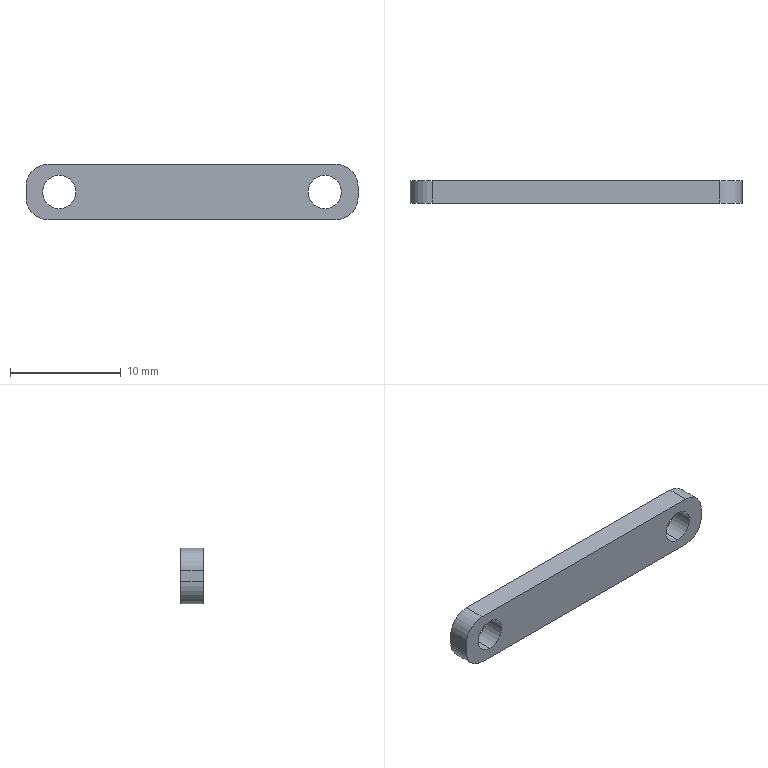Part | SolidWorks | features Extrusion 1 | 1 solid | 14 faces | box 30 x 2 x 5 mm | volume 264.858 mm3 | cylinder 8 | plane 6 | commonest cylinder face diameters 3 x4 4 x4
STEP:
#1=CARTESIAN_POINT('',(-12.,2.,-1.5));
#2=VERTEX_POINT('',#1);
#3=CARTESIAN_POINT('',(-12.,2.,1.5));
#4=VERTEX_POINT('',#3);
#5=CARTESIAN_POINT('',(-12.,2.,0.));
#6=DIRECTION('',(0.,1.,0.));
#7=DIRECTION('',(0.,0.,1.));
#8=AXIS2_PLACEMENT_3D('',#5,#6,#7);
#9=CIRCLE('',#8,1.5);
#10=EDGE_CURVE('',#2,#4,#9,.T.);
#11=ORIENTED_EDGE('',*,*,#10,.T.);
#12=CARTESIAN_POINT('',(-12.,0.,1.5));
#13=VERTEX_POINT('',#12);
#14=CARTESIAN_POINT('',(-12.,2.,1.5));
#15=DIRECTION('',(0.,-1.,0.));
#16=VECTOR('',#15,1000.);
#17=LINE('',#14,#16);
#18=EDGE_CURVE('',#4,#13,#17,.T.);
#19=ORIENTED_EDGE('',*,*,#18,.T.);
#20=CARTESIAN_POINT('',(-12.,0.,-1.5));
#21=VERTEX_POINT('',#20);
#22=CARTESIAN_POINT('',(-12.,0.,0.));
#23=DIRECTION('',(0.,1.,0.));
#24=DIRECTION('',(0.,0.,1.));
#25=AXIS2_PLACEMENT_3D('',#22,#23,#24);
#26=CIRCLE('',#25,1.5);
#27=EDGE_CURVE('',#21,#13,#26,.T.);
#28=ORIENTED_EDGE('',*,*,#27,.F.);
#29=CARTESIAN_POINT('',(-12.,2.,-1.5));
#30=DIRECTION('',(0.,-1.,0.));
#31=VECTOR('',#30,1000.);
#32=LINE('',#29,#31);
#33=EDGE_CURVE('',#2,#21,#32,.T.);
#34=ORIENTED_EDGE('',*,*,#33,.F.);
#35=EDGE_LOOP('',(#11,#19,#28,#34));
#36=FACE_OUTER_BOUND('',#35,.T.);
#37=CARTESIAN_POINT('',(-12.,2.,0.));
#38=DIRECTION('',(0.,-1.,0.));
#39=DIRECTION('',(0.,0.,-1.));
#40=AXIS2_PLACEMENT_3D('',#37,#38,#39);
#41=CYLINDRICAL_SURFACE('',#40,1.5);
#42=ADVANCED_FACE('',(#36),#41,.F.);
#43=CARTESIAN_POINT('',(12.,2.,-1.5));
#44=VERTEX_POINT('',#43);
#45=CARTESIAN_POINT('',(12.,2.,1.5));
#46=VERTEX_POINT('',#45);
#47=CARTESIAN_POINT('',(12.,2.,0.));
#48=DIRECTION('',(0.,1.,0.));
#49=DIRECTION('',(0.,0.,1.));
#50=AXIS2_PLACEMENT_3D('',#47,#48,#49);
#51=CIRCLE('',#50,1.5);
#52=EDGE_CURVE('',#44,#46,#51,.T.);
#53=ORIENTED_EDGE('',*,*,#52,.T.);
#54=CARTESIAN_POINT('',(12.,0.,1.5));
#55=VERTEX_POINT('',#54);
#56=CARTESIAN_POINT('',(12.,2.,1.5));
#57=DIRECTION('',(0.,-1.,0.));
#58=VECTOR('',#57,1000.);
#59=LINE('',#56,#58);
#60=EDGE_CURVE('',#46,#55,#59,.T.);
#61=ORIENTED_EDGE('',*,*,#60,.T.);
#62=CARTESIAN_POINT('',(12.,0.,-1.5));
#63=VERTEX_POINT('',#62);
#64=CARTESIAN_POINT('',(12.,0.,0.));
#65=DIRECTION('',(0.,1.,0.));
#66=DIRECTION('',(0.,0.,1.));
#67=AXIS2_PLACEMENT_3D('',#64,#65,#66);
#68=CIRCLE('',#67,1.5);
#69=EDGE_CURVE('',#63,#55,#68,.T.);
#70=ORIENTED_EDGE('',*,*,#69,.F.);
#71=CARTESIAN_POINT('',(12.,2.,-1.5));
#72=DIRECTION('',(0.,-1.,0.));
#73=VECTOR('',#72,1000.);
#74=LINE('',#71,#73);
#75=EDGE_CURVE('',#44,#63,#74,.T.);
#76=ORIENTED_EDGE('',*,*,#75,.F.);
#77=EDGE_LOOP('',(#53,#61,#70,#76));
#78=FACE_OUTER_BOUND('',#77,.T.);
#79=CARTESIAN_POINT('',(12.,2.,0.));
#80=DIRECTION('',(0.,-1.,0.));
#81=DIRECTION('',(0.,0.,-1.));
#82=AXIS2_PLACEMENT_3D('',#79,#80,#81);
#83=CYLINDRICAL_SURFACE('',#82,1.5);
#84=ADVANCED_FACE('',(#78),#83,.F.);
#85=ORIENTED_EDGE('',*,*,#52,.F.);
#86=CARTESIAN_POINT('',(12.,2.,0.));
#87=DIRECTION('',(0.,1.,0.));
#88=DIRECTION('',(0.,0.,1.));
#89=AXIS2_PLACEMENT_3D('',#86,#87,#88);
#90=CIRCLE('',#89,1.5);
#91=EDGE_CURVE('',#46,#44,#90,.T.);
#92=ORIENTED_EDGE('',*,*,#91,.F.);
#93=EDGE_LOOP('',(#85,#92));
#94=FACE_BOUND('',#93,.T.);
#95=CARTESIAN_POINT('',(15.,2.,-0.5));
#96=VERTEX_POINT('',#95);
#97=CARTESIAN_POINT('',(13.,2.,-2.5));
#98=VERTEX_POINT('',#97);
#99=CARTESIAN_POINT('',(13.,2.,-0.5));
#100=DIRECTION('',(0.,1.,0.));
#101=DIRECTION('',(0.,0.,1.));
#102=AXIS2_PLACEMENT_3D('',#99,#100,#101);
#103=CIRCLE('',#102,2.);
#104=EDGE_CURVE('',#96,#98,#103,.T.);
#105=ORIENTED_EDGE('',*,*,#104,.T.);
#106=CARTESIAN_POINT('',(-13.,2.,-2.5));
#107=VERTEX_POINT('',#106);
#108=CARTESIAN_POINT('',(-13.,2.,-2.5));
#109=DIRECTION('',(-1.,0.,0.));
#110=VECTOR('',#109,1000.);
#111=LINE('',#108,#110);
#112=EDGE_CURVE('',#98,#107,#111,.T.);
#113=ORIENTED_EDGE('',*,*,#112,.T.);
#114=CARTESIAN_POINT('',(-15.,2.,-0.5));
#115=VERTEX_POINT('',#114);
#116=CARTESIAN_POINT('',(-13.,2.,-0.5));
#117=DIRECTION('',(0.,1.,0.));
#118=DIRECTION('',(0.,0.,-1.));
#119=AXIS2_PLACEMENT_3D('',#116,#117,#118);
#120=CIRCLE('',#119,2.);
#121=EDGE_CURVE('',#107,#115,#120,.T.);
#122=ORIENTED_EDGE('',*,*,#121,.T.);
#123=CARTESIAN_POINT('',(-15.,2.,0.5));
#124=VERTEX_POINT('',#123);
#125=CARTESIAN_POINT('',(-15.,2.,0.5));
#126=DIRECTION('',(0.,0.,1.));
#127=VECTOR('',#126,1000.);
#128=LINE('',#125,#127);
#129=EDGE_CURVE('',#115,#124,#128,.T.);
#130=ORIENTED_EDGE('',*,*,#129,.T.);
#131=CARTESIAN_POINT('',(-13.,2.,2.5));
#132=VERTEX_POINT('',#131);
#133=CARTESIAN_POINT('',(-13.,2.,0.5));
#134=DIRECTION('',(0.,1.,0.));
#135=DIRECTION('',(0.,0.,-1.));
#136=AXIS2_PLACEMENT_3D('',#133,#134,#135);
#137=CIRCLE('',#136,2.);
#138=EDGE_CURVE('',#124,#132,#137,.T.);
#139=ORIENTED_EDGE('',*,*,#138,.T.);
#140=CARTESIAN_POINT('',(13.,2.,2.5));
#141=VERTEX_POINT('',#140);
#142=CARTESIAN_POINT('',(-13.,2.,2.5));
#143=DIRECTION('',(1.,0.,0.));
#144=VECTOR('',#143,1000.);
#145=LINE('',#142,#144);
#146=EDGE_CURVE('',#132,#141,#145,.T.);
#147=ORIENTED_EDGE('',*,*,#146,.T.);
#148=CARTESIAN_POINT('',(15.,2.,0.5));
#149=VERTEX_POINT('',#148);
#150=CARTESIAN_POINT('',(13.,2.,0.5));
#151=DIRECTION('',(0.,1.,0.));
#152=DIRECTION('',(0.,0.,-1.));
#153=AXIS2_PLACEMENT_3D('',#150,#151,#152);
#154=CIRCLE('',#153,2.);
#155=EDGE_CURVE('',#141,#149,#154,.T.);
#156=ORIENTED_EDGE('',*,*,#155,.T.);
#157=CARTESIAN_POINT('',(15.,2.,0.5));
#158=DIRECTION('',(0.,0.,-1.));
#159=VECTOR('',#158,1000.);
#160=LINE('',#157,#159);
#161=EDGE_CURVE('',#149,#96,#160,.T.);
#162=ORIENTED_EDGE('',*,*,#161,.T.);
#163=EDGE_LOOP('',(#105,#113,#122,#130,#139,#147,#156,#162));
#164=FACE_OUTER_BOUND('',#163,.T.);
#165=ORIENTED_EDGE('',*,*,#10,.F.);
#166=CARTESIAN_POINT('',(-12.,2.,0.));
#167=DIRECTION('',(0.,1.,0.));
#168=DIRECTION('',(0.,0.,1.));
#169=AXIS2_PLACEMENT_3D('',#166,#167,#168);
#170=CIRCLE('',#169,1.5);
#171=EDGE_CURVE('',#4,#2,#170,.T.);
#172=ORIENTED_EDGE('',*,*,#171,.F.);
#173=EDGE_LOOP('',(#165,#172));
#174=FACE_BOUND('',#173,.T.);
#175=CARTESIAN_POINT('',(13.,2.,-0.5));
#176=DIRECTION('',(0.,1.,0.));
#177=DIRECTION('',(0.,0.,1.));
#178=AXIS2_PLACEMENT_3D('',#175,#176,#177);
#179=PLANE('',#178);
#180=ADVANCED_FACE('',(#94,#164,#174),#179,.T.);
#181=CARTESIAN_POINT('',(15.,0.,-0.5));
#182=VERTEX_POINT('',#181);
#183=CARTESIAN_POINT('',(13.,0.,-2.5));
#184=VERTEX_POINT('',#183);
#185=CARTESIAN_POINT('',(13.,0.,-0.5));
#186=DIRECTION('',(0.,1.,0.));
#187=DIRECTION('',(0.,0.,1.));
#188=AXIS2_PLACEMENT_3D('',#185,#186,#187);
#189=CIRCLE('',#188,2.);
#190=EDGE_CURVE('',#182,#184,#189,.T.);
#191=ORIENTED_EDGE('',*,*,#190,.F.);
#192=CARTESIAN_POINT('',(15.,0.,0.5));
#193=VERTEX_POINT('',#192);
#194=CARTESIAN_POINT('',(15.,0.,0.5));
#195=DIRECTION('',(0.,0.,-1.));
#196=VECTOR('',#195,1000.);
#197=LINE('',#194,#196);
#198=EDGE_CURVE('',#193,#182,#197,.T.);
#199=ORIENTED_EDGE('',*,*,#198,.F.);
#200=CARTESIAN_POINT('',(13.,0.,2.5));
#201=VERTEX_POINT('',#200);
#202=CARTESIAN_POINT('',(13.,0.,0.5));
#203=DIRECTION('',(0.,1.,0.));
#204=DIRECTION('',(0.,0.,-1.));
#205=AXIS2_PLACEMENT_3D('',#202,#203,#204);
#206=CIRCLE('',#205,2.);
#207=EDGE_CURVE('',#201,#193,#206,.T.);
#208=ORIENTED_EDGE('',*,*,#207,.F.);
#209=CARTESIAN_POINT('',(-13.,0.,2.5));
#210=VERTEX_POINT('',#209);
#211=CARTESIAN_POINT('',(-13.,0.,2.5));
#212=DIRECTION('',(1.,0.,0.));
#213=VECTOR('',#212,1000.);
#214=LINE('',#211,#213);
#215=EDGE_CURVE('',#210,#201,#214,.T.);
#216=ORIENTED_EDGE('',*,*,#215,.F.);
#217=CARTESIAN_POINT('',(-15.,0.,0.5));
#218=VERTEX_POINT('',#217);
#219=CARTESIAN_POINT('',(-13.,0.,0.5));
#220=DIRECTION('',(0.,1.,0.));
#221=DIRECTION('',(0.,0.,-1.));
#222=AXIS2_PLACEMENT_3D('',#219,#220,#221);
#223=CIRCLE('',#222,2.);
#224=EDGE_CURVE('',#218,#210,#223,.T.);
#225=ORIENTED_EDGE('',*,*,#224,.F.);
#226=CARTESIAN_POINT('',(-15.,0.,-0.5));
#227=VERTEX_POINT('',#226);
#228=CARTESIAN_POINT('',(-15.,0.,0.5));
#229=DIRECTION('',(0.,0.,1.));
#230=VECTOR('',#229,1000.);
#231=LINE('',#228,#230);
#232=EDGE_CURVE('',#227,#218,#231,.T.);
#233=ORIENTED_EDGE('',*,*,#232,.F.);
#234=CARTESIAN_POINT('',(-13.,0.,-2.5));
#235=VERTEX_POINT('',#234);
#236=CARTESIAN_POINT('',(-13.,0.,-0.5));
#237=DIRECTION('',(0.,1.,0.));
#238=DIRECTION('',(0.,0.,-1.));
#239=AXIS2_PLACEMENT_3D('',#236,#237,#238);
#240=CIRCLE('',#239,2.);
#241=EDGE_CURVE('',#235,#227,#240,.T.);
#242=ORIENTED_EDGE('',*,*,#241,.F.);
#243=CARTESIAN_POINT('',(-13.,0.,-2.5));
#244=DIRECTION('',(-1.,0.,0.));
#245=VECTOR('',#244,1000.);
#246=LINE('',#243,#245);
#247=EDGE_CURVE('',#184,#235,#246,.T.);
#248=ORIENTED_EDGE('',*,*,#247,.F.);
#249=EDGE_LOOP('',(#191,#199,#208,#216,#225,#233,#242,#248));
#250=FACE_OUTER_BOUND('',#249,.T.);
#251=ORIENTED_EDGE('',*,*,#69,.T.);
#252=CARTESIAN_POINT('',(12.,0.,0.));
#253=DIRECTION('',(0.,1.,0.));
#254=DIRECTION('',(0.,0.,1.));
#255=AXIS2_PLACEMENT_3D('',#252,#253,#254);
#256=CIRCLE('',#255,1.5);
#257=EDGE_CURVE('',#55,#63,#256,.T.);
#258=ORIENTED_EDGE('',*,*,#257,.T.);
#259=EDGE_LOOP('',(#251,#258));
#260=FACE_BOUND('',#259,.T.);
#261=ORIENTED_EDGE('',*,*,#27,.T.);
#262=CARTESIAN_POINT('',(-12.,0.,0.));
#263=DIRECTION('',(0.,1.,0.));
#264=DIRECTION('',(0.,0.,1.));
#265=AXIS2_PLACEMENT_3D('',#262,#263,#264);
#266=CIRCLE('',#265,1.5);
#267=EDGE_CURVE('',#13,#21,#266,.T.);
#268=ORIENTED_EDGE('',*,*,#267,.T.);
#269=EDGE_LOOP('',(#261,#268));
#270=FACE_BOUND('',#269,.T.);
#271=CARTESIAN_POINT('',(13.,0.,-0.5));
#272=DIRECTION('',(0.,1.,0.));
#273=DIRECTION('',(0.,0.,1.));
#274=AXIS2_PLACEMENT_3D('',#271,#272,#273);
#275=PLANE('',#274);
#276=ADVANCED_FACE('',(#250,#260,#270),#275,.F.);
#277=ORIENTED_EDGE('',*,*,#190,.T.);
#278=CARTESIAN_POINT('',(13.,2.,-2.5));
#279=DIRECTION('',(0.,-1.,0.));
#280=VECTOR('',#279,1000.);
#281=LINE('',#278,#280);
#282=EDGE_CURVE('',#98,#184,#281,.T.);
#283=ORIENTED_EDGE('',*,*,#282,.F.);
#284=ORIENTED_EDGE('',*,*,#104,.F.);
#285=CARTESIAN_POINT('',(15.,2.,-0.5));
#286=DIRECTION('',(0.,-1.,0.));
#287=VECTOR('',#286,1000.);
#288=LINE('',#285,#287);
#289=EDGE_CURVE('',#96,#182,#288,.T.);
#290=ORIENTED_EDGE('',*,*,#289,.T.);
#291=EDGE_LOOP('',(#277,#283,#284,#290));
#292=FACE_OUTER_BOUND('',#291,.T.);
#293=CARTESIAN_POINT('',(13.,2.,-0.5));
#294=DIRECTION('',(0.,-1.,0.));
#295=DIRECTION('',(0.,0.,-1.));
#296=AXIS2_PLACEMENT_3D('',#293,#294,#295);
#297=CYLINDRICAL_SURFACE('',#296,2.);
#298=ADVANCED_FACE('',(#292),#297,.T.);
#299=ORIENTED_EDGE('',*,*,#247,.T.);
#300=CARTESIAN_POINT('',(-13.,2.,-2.5));
#301=DIRECTION('',(0.,-1.,0.));
#302=VECTOR('',#301,1000.);
#303=LINE('',#300,#302);
#304=EDGE_CURVE('',#107,#235,#303,.T.);
#305=ORIENTED_EDGE('',*,*,#304,.F.);
#306=ORIENTED_EDGE('',*,*,#112,.F.);
#307=ORIENTED_EDGE('',*,*,#282,.T.);
#308=EDGE_LOOP('',(#299,#305,#306,#307));
#309=FACE_OUTER_BOUND('',#308,.T.);
#310=CARTESIAN_POINT('',(-13.,2.,-2.5));
#311=DIRECTION('',(0.,0.,1.));
#312=DIRECTION('',(1.,0.,0.));
#313=AXIS2_PLACEMENT_3D('',#310,#311,#312);
#314=PLANE('',#313);
#315=ADVANCED_FACE('',(#309),#314,.F.);
#316=ORIENTED_EDGE('',*,*,#241,.T.);
#317=CARTESIAN_POINT('',(-15.,2.,-0.5));
#318=DIRECTION('',(0.,-1.,0.));
#319=VECTOR('',#318,1000.);
#320=LINE('',#317,#319);
#321=EDGE_CURVE('',#115,#227,#320,.T.);
#322=ORIENTED_EDGE('',*,*,#321,.F.);
#323=ORIENTED_EDGE('',*,*,#121,.F.);
#324=ORIENTED_EDGE('',*,*,#304,.T.);
#325=EDGE_LOOP('',(#316,#322,#323,#324));
#326=FACE_OUTER_BOUND('',#325,.T.);
#327=CARTESIAN_POINT('',(-13.,2.,-0.5));
#328=DIRECTION('',(0.,-1.,0.));
#329=DIRECTION('',(0.,0.,-1.));
#330=AXIS2_PLACEMENT_3D('',#327,#328,#329);
#331=CYLINDRICAL_SURFACE('',#330,2.);
#332=ADVANCED_FACE('',(#326),#331,.T.);
#333=ORIENTED_EDGE('',*,*,#232,.T.);
#334=CARTESIAN_POINT('',(-15.,2.,0.5));
#335=DIRECTION('',(0.,-1.,0.));
#336=VECTOR('',#335,1000.);
#337=LINE('',#334,#336);
#338=EDGE_CURVE('',#124,#218,#337,.T.);
#339=ORIENTED_EDGE('',*,*,#338,.F.);
#340=ORIENTED_EDGE('',*,*,#129,.F.);
#341=ORIENTED_EDGE('',*,*,#321,.T.);
#342=EDGE_LOOP('',(#333,#339,#340,#341));
#343=FACE_OUTER_BOUND('',#342,.T.);
#344=CARTESIAN_POINT('',(-15.,2.,0.5));
#345=DIRECTION('',(1.,0.,0.));
#346=DIRECTION('',(0.,0.,-1.));
#347=AXIS2_PLACEMENT_3D('',#344,#345,#346);
#348=PLANE('',#347);
#349=ADVANCED_FACE('',(#343),#348,.F.);
#350=ORIENTED_EDGE('',*,*,#224,.T.);
#351=CARTESIAN_POINT('',(-13.,2.,2.5));
#352=DIRECTION('',(0.,-1.,0.));
#353=VECTOR('',#352,1000.);
#354=LINE('',#351,#353);
#355=EDGE_CURVE('',#132,#210,#354,.T.);
#356=ORIENTED_EDGE('',*,*,#355,.F.);
#357=ORIENTED_EDGE('',*,*,#138,.F.);
#358=ORIENTED_EDGE('',*,*,#338,.T.);
#359=EDGE_LOOP('',(#350,#356,#357,#358));
#360=FACE_OUTER_BOUND('',#359,.T.);
#361=CARTESIAN_POINT('',(-13.,2.,0.5));
#362=DIRECTION('',(0.,-1.,0.));
#363=DIRECTION('',(0.,0.,-1.));
#364=AXIS2_PLACEMENT_3D('',#361,#362,#363);
#365=CYLINDRICAL_SURFACE('',#364,2.);
#366=ADVANCED_FACE('',(#360),#365,.T.);
#367=ORIENTED_EDGE('',*,*,#215,.T.);
#368=CARTESIAN_POINT('',(13.,2.,2.5));
#369=DIRECTION('',(0.,-1.,0.));
#370=VECTOR('',#369,1000.);
#371=LINE('',#368,#370);
#372=EDGE_CURVE('',#141,#201,#371,.T.);
#373=ORIENTED_EDGE('',*,*,#372,.F.);
#374=ORIENTED_EDGE('',*,*,#146,.F.);
#375=ORIENTED_EDGE('',*,*,#355,.T.);
#376=EDGE_LOOP('',(#367,#373,#374,#375));
#377=FACE_OUTER_BOUND('',#376,.T.);
#378=CARTESIAN_POINT('',(-13.,2.,2.5));
#379=DIRECTION('',(0.,0.,-1.));
#380=DIRECTION('',(-1.,0.,0.));
#381=AXIS2_PLACEMENT_3D('',#378,#379,#380);
#382=PLANE('',#381);
#383=ADVANCED_FACE('',(#377),#382,.F.);
#384=ORIENTED_EDGE('',*,*,#207,.T.);
#385=CARTESIAN_POINT('',(15.,2.,0.5));
#386=DIRECTION('',(0.,-1.,0.));
#387=VECTOR('',#386,1000.);
#388=LINE('',#385,#387);
#389=EDGE_CURVE('',#149,#193,#388,.T.);
#390=ORIENTED_EDGE('',*,*,#389,.F.);
#391=ORIENTED_EDGE('',*,*,#155,.F.);
#392=ORIENTED_EDGE('',*,*,#372,.T.);
#393=EDGE_LOOP('',(#384,#390,#391,#392));
#394=FACE_OUTER_BOUND('',#393,.T.);
#395=CARTESIAN_POINT('',(13.,2.,0.5));
#396=DIRECTION('',(0.,-1.,0.));
#397=DIRECTION('',(0.,0.,-1.));
#398=AXIS2_PLACEMENT_3D('',#395,#396,#397);
#399=CYLINDRICAL_SURFACE('',#398,2.);
#400=ADVANCED_FACE('',(#394),#399,.T.);
#401=ORIENTED_EDGE('',*,*,#198,.T.);
#402=ORIENTED_EDGE('',*,*,#289,.F.);
#403=ORIENTED_EDGE('',*,*,#161,.F.);
#404=ORIENTED_EDGE('',*,*,#389,.T.);
#405=EDGE_LOOP('',(#401,#402,#403,#404));
#406=FACE_OUTER_BOUND('',#405,.T.);
#407=CARTESIAN_POINT('',(15.,2.,0.5));
#408=DIRECTION('',(-1.,0.,0.));
#409=DIRECTION('',(0.,0.,1.));
#410=AXIS2_PLACEMENT_3D('',#407,#408,#409);
#411=PLANE('',#410);
#412=ADVANCED_FACE('',(#406),#411,.F.);
#413=ORIENTED_EDGE('',*,*,#60,.F.);
#414=ORIENTED_EDGE('',*,*,#91,.T.);
#415=ORIENTED_EDGE('',*,*,#75,.T.);
#416=ORIENTED_EDGE('',*,*,#257,.F.);
#417=EDGE_LOOP('',(#413,#414,#415,#416));
#418=FACE_OUTER_BOUND('',#417,.T.);
#419=CARTESIAN_POINT('',(12.,2.,0.));
#420=DIRECTION('',(0.,-1.,0.));
#421=DIRECTION('',(0.,0.,-1.));
#422=AXIS2_PLACEMENT_3D('',#419,#420,#421);
#423=CYLINDRICAL_SURFACE('',#422,1.5);
#424=ADVANCED_FACE('',(#418),#423,.F.);
#425=ORIENTED_EDGE('',*,*,#18,.F.);
#426=ORIENTED_EDGE('',*,*,#171,.T.);
#427=ORIENTED_EDGE('',*,*,#33,.T.);
#428=ORIENTED_EDGE('',*,*,#267,.F.);
#429=EDGE_LOOP('',(#425,#426,#427,#428));
#430=FACE_OUTER_BOUND('',#429,.T.);
#431=CARTESIAN_POINT('',(-12.,2.,0.));
#432=DIRECTION('',(0.,-1.,0.));
#433=DIRECTION('',(0.,0.,-1.));
#434=AXIS2_PLACEMENT_3D('',#431,#432,#433);
#435=CYLINDRICAL_SURFACE('',#434,1.5);
#436=ADVANCED_FACE('',(#430),#435,.F.);
#437=CLOSED_SHELL('',(#42,#84,#180,#276,#298,#315,#332,#349,#366,#383,#400,#412,#424,#436));
#438=MANIFOLD_SOLID_BREP('',#437);
#439=CARTESIAN_POINT('',(0.,0.,0.));
#440=DIRECTION('',(0.,0.,1.));
#441=DIRECTION('',(1.,0.,0.));
#442=AXIS2_PLACEMENT_3D('',#439,#440,#441);
#443=(LENGTH_UNIT()NAMED_UNIT(*)SI_UNIT(.MILLI.,.METRE.));
#444=UNCERTAINTY_MEASURE_WITH_UNIT(LENGTH_MEASURE(0.00001),#443,'','');
#445=(NAMED_UNIT(*)PLANE_ANGLE_UNIT()SI_UNIT($,.RADIAN.));
#446=(NAMED_UNIT(*)SI_UNIT($,.STERADIAN.)SOLID_ANGLE_UNIT());
#447=(GEOMETRIC_REPRESENTATION_CONTEXT(3)GLOBAL_UNCERTAINTY_ASSIGNED_CONTEXT((#444))GLOBAL_UNIT_ASSIGNED_CONTEXT((#443,#445,#446))REPRESENTATION_CONTEXT('',''));
#448=ADVANCED_BREP_SHAPE_REPRESENTATION('',(#438,#442),#447);